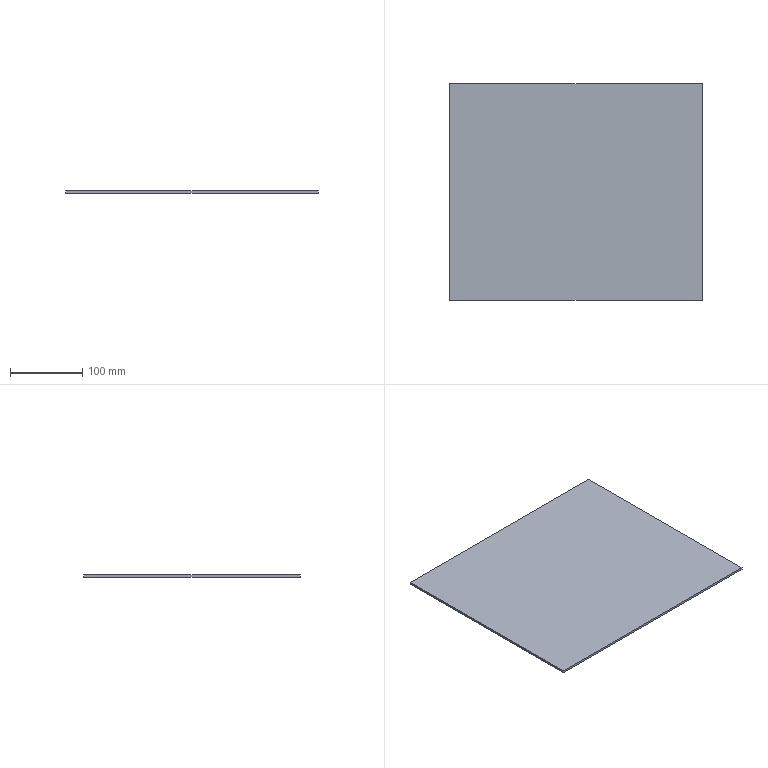Part | NX | features stopper partition 2 | 1 solid | 6 faces | box 350 x 300 x 3 mm | volume 315000 mm3 | plane 6
STEP:
#1=CARTESIAN_POINT('',(-175.,0.,0.));
#2=VERTEX_POINT('',#1);
#3=CARTESIAN_POINT('',(-175.,300.,0.));
#4=VERTEX_POINT('',#3);
#5=CARTESIAN_POINT('',(-175.,0.,0.));
#6=DIRECTION('',(0.,1.,0.));
#7=VECTOR('',#6,1000.);
#8=LINE('',#5,#7);
#9=EDGE_CURVE('',#2,#4,#8,.T.);
#10=ORIENTED_EDGE('',*,*,#9,.T.);
#11=CARTESIAN_POINT('',(175.,300.,0.));
#12=VERTEX_POINT('',#11);
#13=CARTESIAN_POINT('',(-175.,300.,0.));
#14=DIRECTION('',(1.,0.,0.));
#15=VECTOR('',#14,1000.);
#16=LINE('',#13,#15);
#17=EDGE_CURVE('',#4,#12,#16,.T.);
#18=ORIENTED_EDGE('',*,*,#17,.T.);
#19=CARTESIAN_POINT('',(175.,0.,0.));
#20=VERTEX_POINT('',#19);
#21=CARTESIAN_POINT('',(175.,0.,0.));
#22=DIRECTION('',(0.,1.,0.));
#23=VECTOR('',#22,1000.);
#24=LINE('',#21,#23);
#25=EDGE_CURVE('',#12,#20,#24,.F.);
#26=ORIENTED_EDGE('',*,*,#25,.T.);
#27=CARTESIAN_POINT('',(-175.,0.,0.));
#28=DIRECTION('',(1.,0.,0.));
#29=VECTOR('',#28,1000.);
#30=LINE('',#27,#29);
#31=EDGE_CURVE('',#20,#2,#30,.F.);
#32=ORIENTED_EDGE('',*,*,#31,.T.);
#33=EDGE_LOOP('',(#10,#18,#26,#32));
#34=FACE_BOUND('',#33,.T.);
#35=CARTESIAN_POINT('',(175.,300.,0.));
#36=DIRECTION('',(0.,0.,-1.));
#37=DIRECTION('',(-1.,0.,0.));
#38=AXIS2_PLACEMENT_3D('',#35,#36,#37);
#39=PLANE('',#38);
#40=ADVANCED_FACE('',(#34),#39,.T.);
#41=CARTESIAN_POINT('',(175.,0.,3.));
#42=VERTEX_POINT('',#41);
#43=CARTESIAN_POINT('',(175.,0.,3.));
#44=DIRECTION('',(0.,0.,1.));
#45=VECTOR('',#44,1000.);
#46=LINE('',#43,#45);
#47=EDGE_CURVE('',#20,#42,#46,.T.);
#48=ORIENTED_EDGE('',*,*,#47,.T.);
#49=CARTESIAN_POINT('',(-175.,0.,3.));
#50=VERTEX_POINT('',#49);
#51=CARTESIAN_POINT('',(175.,0.,3.));
#52=DIRECTION('',(-1.,0.,0.));
#53=VECTOR('',#52,1000.);
#54=LINE('',#51,#53);
#55=EDGE_CURVE('',#42,#50,#54,.T.);
#56=ORIENTED_EDGE('',*,*,#55,.T.);
#57=CARTESIAN_POINT('',(-175.,0.,3.));
#58=DIRECTION('',(0.,0.,-1.));
#59=VECTOR('',#58,1000.);
#60=LINE('',#57,#59);
#61=EDGE_CURVE('',#50,#2,#60,.T.);
#62=ORIENTED_EDGE('',*,*,#61,.T.);
#63=ORIENTED_EDGE('',*,*,#31,.F.);
#64=EDGE_LOOP('',(#48,#56,#62,#63));
#65=FACE_BOUND('',#64,.T.);
#66=CARTESIAN_POINT('',(-175.,0.,3.));
#67=DIRECTION('',(0.,1.,0.));
#68=DIRECTION('',(0.,0.,1.));
#69=AXIS2_PLACEMENT_3D('',#66,#67,#68);
#70=PLANE('',#69);
#71=ADVANCED_FACE('',(#65),#70,.F.);
#72=ORIENTED_EDGE('',*,*,#61,.F.);
#73=CARTESIAN_POINT('',(-175.,300.,3.));
#74=VERTEX_POINT('',#73);
#75=CARTESIAN_POINT('',(-175.,300.,3.));
#76=DIRECTION('',(0.,1.,0.));
#77=VECTOR('',#76,1000.);
#78=LINE('',#75,#77);
#79=EDGE_CURVE('',#50,#74,#78,.T.);
#80=ORIENTED_EDGE('',*,*,#79,.T.);
#81=CARTESIAN_POINT('',(-175.,300.,3.));
#82=DIRECTION('',(0.,0.,-1.));
#83=VECTOR('',#82,1000.);
#84=LINE('',#81,#83);
#85=EDGE_CURVE('',#74,#4,#84,.T.);
#86=ORIENTED_EDGE('',*,*,#85,.T.);
#87=ORIENTED_EDGE('',*,*,#9,.F.);
#88=EDGE_LOOP('',(#72,#80,#86,#87));
#89=FACE_BOUND('',#88,.T.);
#90=CARTESIAN_POINT('',(-175.,0.,3.));
#91=DIRECTION('',(1.,0.,0.));
#92=DIRECTION('',(0.,0.,-1.));
#93=AXIS2_PLACEMENT_3D('',#90,#91,#92);
#94=PLANE('',#93);
#95=ADVANCED_FACE('',(#89),#94,.F.);
#96=ORIENTED_EDGE('',*,*,#85,.F.);
#97=CARTESIAN_POINT('',(175.,300.,3.));
#98=VERTEX_POINT('',#97);
#99=CARTESIAN_POINT('',(175.,300.,3.));
#100=DIRECTION('',(-1.,0.,0.));
#101=VECTOR('',#100,1000.);
#102=LINE('',#99,#101);
#103=EDGE_CURVE('',#74,#98,#102,.F.);
#104=ORIENTED_EDGE('',*,*,#103,.T.);
#105=CARTESIAN_POINT('',(175.,300.,3.));
#106=DIRECTION('',(0.,0.,1.));
#107=VECTOR('',#106,1000.);
#108=LINE('',#105,#107);
#109=EDGE_CURVE('',#98,#12,#108,.F.);
#110=ORIENTED_EDGE('',*,*,#109,.T.);
#111=ORIENTED_EDGE('',*,*,#17,.F.);
#112=EDGE_LOOP('',(#96,#104,#110,#111));
#113=FACE_BOUND('',#112,.T.);
#114=CARTESIAN_POINT('',(-175.,300.,3.));
#115=DIRECTION('',(0.,-1.,0.));
#116=DIRECTION('',(0.,0.,-1.));
#117=AXIS2_PLACEMENT_3D('',#114,#115,#116);
#118=PLANE('',#117);
#119=ADVANCED_FACE('',(#113),#118,.F.);
#120=ORIENTED_EDGE('',*,*,#109,.F.);
#121=CARTESIAN_POINT('',(175.,300.,3.));
#122=DIRECTION('',(0.,1.,0.));
#123=VECTOR('',#122,1000.);
#124=LINE('',#121,#123);
#125=EDGE_CURVE('',#98,#42,#124,.F.);
#126=ORIENTED_EDGE('',*,*,#125,.T.);
#127=ORIENTED_EDGE('',*,*,#47,.F.);
#128=ORIENTED_EDGE('',*,*,#25,.F.);
#129=EDGE_LOOP('',(#120,#126,#127,#128));
#130=FACE_BOUND('',#129,.T.);
#131=CARTESIAN_POINT('',(175.,0.,3.));
#132=DIRECTION('',(-1.,0.,0.));
#133=DIRECTION('',(0.,0.,1.));
#134=AXIS2_PLACEMENT_3D('',#131,#132,#133);
#135=PLANE('',#134);
#136=ADVANCED_FACE('',(#130),#135,.F.);
#137=ORIENTED_EDGE('',*,*,#103,.F.);
#138=ORIENTED_EDGE('',*,*,#79,.F.);
#139=ORIENTED_EDGE('',*,*,#55,.F.);
#140=ORIENTED_EDGE('',*,*,#125,.F.);
#141=EDGE_LOOP('',(#137,#138,#139,#140));
#142=FACE_BOUND('',#141,.T.);
#143=CARTESIAN_POINT('',(175.,300.,3.));
#144=DIRECTION('',(0.,0.,-1.));
#145=DIRECTION('',(-1.,0.,0.));
#146=AXIS2_PLACEMENT_3D('',#143,#144,#145);
#147=PLANE('',#146);
#148=ADVANCED_FACE('',(#142),#147,.F.);
#149=CLOSED_SHELL('',(#40,#71,#95,#119,#136,#148));
#150=MANIFOLD_SOLID_BREP('',#149);
#151=(LENGTH_UNIT()NAMED_UNIT(*)SI_UNIT(.MILLI.,.METRE.));
#152=UNCERTAINTY_MEASURE_WITH_UNIT(LENGTH_MEASURE(0.00001),#151,'','');
#153=(NAMED_UNIT(*)PLANE_ANGLE_UNIT()SI_UNIT($,.RADIAN.));
#154=(NAMED_UNIT(*)SI_UNIT($,.STERADIAN.)SOLID_ANGLE_UNIT());
#155=(GEOMETRIC_REPRESENTATION_CONTEXT(3)GLOBAL_UNCERTAINTY_ASSIGNED_CONTEXT((#152))GLOBAL_UNIT_ASSIGNED_CONTEXT((#151,#153,#154))REPRESENTATION_CONTEXT('',''));
#156=ADVANCED_BREP_SHAPE_REPRESENTATION('',(#150),#155);